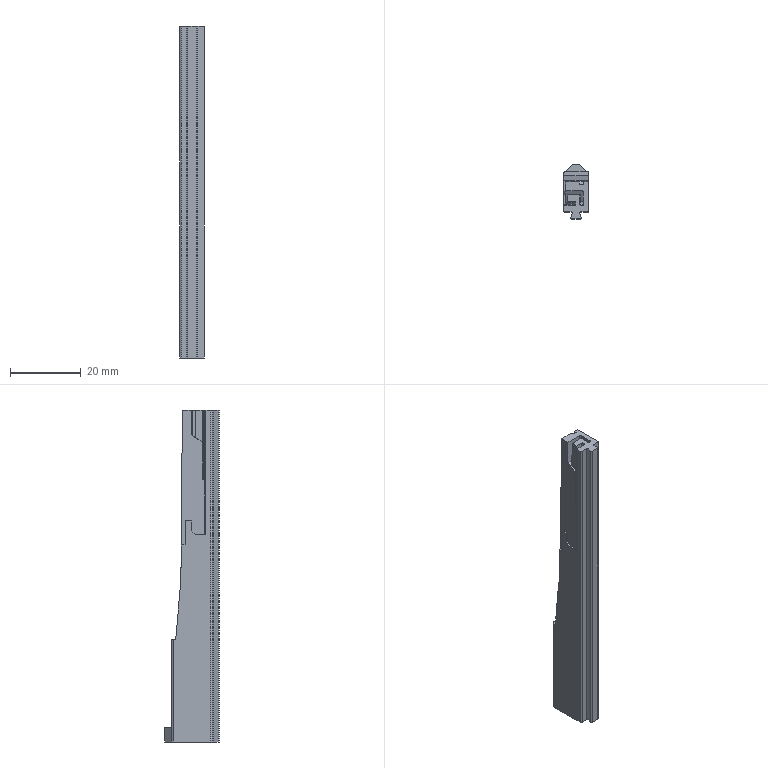Part | Creo | 1 solid | 57 faces | box 7.012 x 15.538 x 94.171 mm | volume 6684 mm3 | plane 43 | cylinder 14 | commonest cylinder face diameters 0.603 x8 0.6 x4 1 x2